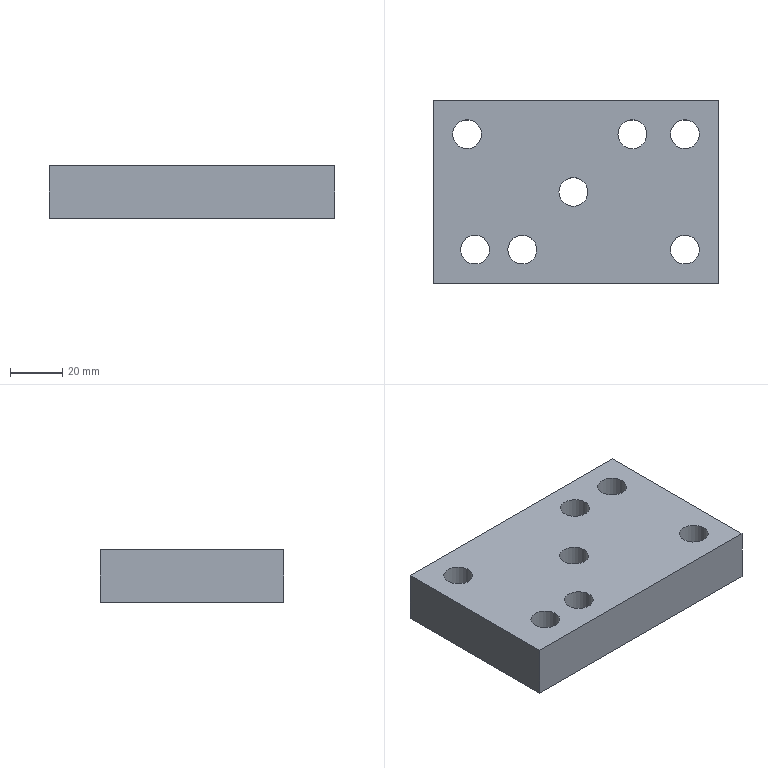Part | STEP file | 115_id2850_x_t | 1 solid | 13 faces | box 109 x 70 x 20 mm | volume 139295 mm3 | cylinder 7 | plane 6 | commonest cylinder face diameters 11 x7
STEP:
#1=CARTESIAN_POINT('',(0.,0.,0.));
#2=DIRECTION('',(0.,0.,1.));
#3=DIRECTION('',(1.,0.,0.));
#4=AXIS2_PLACEMENT_3D('',#1,#2,#3);
#5=CARTESIAN_POINT('',(1035.5,-161.,105.));
#6=VERTEX_POINT('',#5);
#7=CARTESIAN_POINT('',(1030.,-161.,105.));
#8=DIRECTION('',(0.,0.,1.));
#9=DIRECTION('',(1.,0.,0.));
#10=AXIS2_PLACEMENT_3D('',#7,#8,#9);
#11=CIRCLE('',#10,5.5);
#12=CARTESIAN_POINT('',(1030.,-162.5,105.));
#13=DIRECTION('',(0.,0.,1.));
#14=DIRECTION('',(-1.,0.,0.));
#15=AXIS2_PLACEMENT_3D('',#12,#13,#14);
#16=PLANE('',#15);
#17=CARTESIAN_POINT('',(0.,-1.5));
#18=DIRECTION('',(-1.,0.));
#19=AXIS2_PLACEMENT_2D('',#17,#18);
#20=CIRCLE('',#19,5.5);
#21=(GEOMETRIC_REPRESENTATION_CONTEXT(2)PARAMETRIC_REPRESENTATION_CONTEXT()REPRESENTATION_CONTEXT('',''));
#22=DEFINITIONAL_REPRESENTATION('',(#20),#21);
#23=PCURVE('',#16,#22);
#24=CARTESIAN_POINT('',(1030.,-161.,165.));
#25=DIRECTION('',(0.,0.,-1.));
#26=DIRECTION('',(1.,0.,0.));
#27=AXIS2_PLACEMENT_3D('',#24,#25,#26);
#28=CYLINDRICAL_SURFACE('',#27,5.5);
#29=CARTESIAN_POINT('',(6.283,60.));
#30=DIRECTION('',(-1.,0.));
#31=VECTOR('',#30,1.);
#32=LINE('',#29,#31);
#33=(GEOMETRIC_REPRESENTATION_CONTEXT(2)PARAMETRIC_REPRESENTATION_CONTEXT()REPRESENTATION_CONTEXT('',''));
#34=DEFINITIONAL_REPRESENTATION('',(#32),#33);
#35=PCURVE('',#28,#34);
#36=SURFACE_CURVE('',#11,(#23,#35),.PCURVE_S1.);
#37=EDGE_CURVE('',#6,#6,#36,.T.);
#38=ORIENTED_EDGE('',*,*,#37,.F.);
#39=EDGE_LOOP('',(#38));
#40=FACE_BOUND('',#39,.T.);
#41=CARTESIAN_POINT('',(1016.,-183.,105.));
#42=VERTEX_POINT('',#41);
#43=CARTESIAN_POINT('',(1005.,-183.,105.));
#44=VERTEX_POINT('',#43);
#45=CARTESIAN_POINT('',(1010.5,-183.,105.));
#46=DIRECTION('',(0.,0.,-1.));
#47=DIRECTION('',(1.,0.,0.));
#48=AXIS2_PLACEMENT_3D('',#45,#46,#47);
#49=CIRCLE('',#48,5.5);
#50=CARTESIAN_POINT('',(14.,20.5));
#51=CARTESIAN_POINT('',(14.,30.026));
#52=CARTESIAN_POINT('',(22.25,25.263));
#53=CARTESIAN_POINT('',(30.5,20.5));
#54=CARTESIAN_POINT('',(22.25,15.737));
#55=CARTESIAN_POINT('',(14.,10.974));
#56=CARTESIAN_POINT('',(14.,20.5));
#57=(BOUNDED_CURVE()B_SPLINE_CURVE(2,(#50,#51,#52,#53,#54,#55,#56),.UNSPECIFIED.,.T.,.F.)B_SPLINE_CURVE_WITH_KNOTS((1,2,2,2,2,1),(-2.094,0.,2.094,4.189,6.283,8.378),.UNSPECIFIED.)CURVE()GEOMETRIC_REPRESENTATION_ITEM()RATIONAL_B_SPLINE_CURVE((1.,0.5,1.,0.5,1.,0.5,1.))REPRESENTATION_ITEM(''));
#58=(GEOMETRIC_REPRESENTATION_CONTEXT(2)PARAMETRIC_REPRESENTATION_CONTEXT()REPRESENTATION_CONTEXT('',''));
#59=DEFINITIONAL_REPRESENTATION('',(#57),#58);
#60=PCURVE('',#16,#59);
#61=CARTESIAN_POINT('',(1010.5,-183.,90.));
#62=DIRECTION('',(0.,0.,1.));
#63=DIRECTION('',(-1.,0.,0.));
#64=AXIS2_PLACEMENT_3D('',#61,#62,#63);
#65=CYLINDRICAL_SURFACE('',#64,5.5);
#66=CARTESIAN_POINT('',(3.142,15.));
#67=DIRECTION('',(-1.,0.));
#68=VECTOR('',#67,1.);
#69=LINE('',#66,#68);
#70=(GEOMETRIC_REPRESENTATION_CONTEXT(2)PARAMETRIC_REPRESENTATION_CONTEXT()REPRESENTATION_CONTEXT('',''));
#71=DEFINITIONAL_REPRESENTATION('',(#69),#70);
#72=PCURVE('',#65,#71);
#73=SURFACE_CURVE('',#49,(#60,#72),.PCURVE_S1.);
#74=EDGE_CURVE('',#42,#44,#73,.T.);
#75=ORIENTED_EDGE('',*,*,#74,.T.);
#76=CARTESIAN_POINT('',(1010.5,-183.,105.));
#77=DIRECTION('',(0.,0.,-1.));
#78=DIRECTION('',(1.,0.,0.));
#79=AXIS2_PLACEMENT_3D('',#76,#77,#78);
#80=CIRCLE('',#79,5.5);
#81=CARTESIAN_POINT('',(14.,20.5));
#82=CARTESIAN_POINT('',(14.,30.026));
#83=CARTESIAN_POINT('',(22.25,25.263));
#84=CARTESIAN_POINT('',(30.5,20.5));
#85=CARTESIAN_POINT('',(22.25,15.737));
#86=CARTESIAN_POINT('',(14.,10.974));
#87=CARTESIAN_POINT('',(14.,20.5));
#88=(BOUNDED_CURVE()B_SPLINE_CURVE(2,(#81,#82,#83,#84,#85,#86,#87),.UNSPECIFIED.,.T.,.F.)B_SPLINE_CURVE_WITH_KNOTS((1,2,2,2,2,1),(-2.094,0.,2.094,4.189,6.283,8.378),.UNSPECIFIED.)CURVE()GEOMETRIC_REPRESENTATION_ITEM()RATIONAL_B_SPLINE_CURVE((1.,0.5,1.,0.5,1.,0.5,1.))REPRESENTATION_ITEM(''));
#89=(GEOMETRIC_REPRESENTATION_CONTEXT(2)PARAMETRIC_REPRESENTATION_CONTEXT()REPRESENTATION_CONTEXT('',''));
#90=DEFINITIONAL_REPRESENTATION('',(#88),#89);
#91=PCURVE('',#16,#90);
#92=CARTESIAN_POINT('',(9.425,15.));
#93=DIRECTION('',(-1.,0.));
#94=VECTOR('',#93,1.);
#95=LINE('',#92,#94);
#96=(GEOMETRIC_REPRESENTATION_CONTEXT(2)PARAMETRIC_REPRESENTATION_CONTEXT()REPRESENTATION_CONTEXT('',''));
#97=DEFINITIONAL_REPRESENTATION('',(#95),#96);
#98=PCURVE('',#65,#97);
#99=SURFACE_CURVE('',#80,(#91,#98),.PCURVE_S1.);
#100=EDGE_CURVE('',#44,#42,#99,.T.);
#101=ORIENTED_EDGE('',*,*,#100,.T.);
#102=EDGE_LOOP('',(#75,#101));
#103=FACE_BOUND('',#102,.T.);
#104=CARTESIAN_POINT('',(1078.,-139.,105.));
#105=VERTEX_POINT('',#104);
#106=CARTESIAN_POINT('',(1067.,-139.,105.));
#107=VERTEX_POINT('',#106);
#108=CARTESIAN_POINT('',(1072.5,-139.,105.));
#109=DIRECTION('',(0.,0.,-1.));
#110=DIRECTION('',(1.,0.,0.));
#111=AXIS2_PLACEMENT_3D('',#108,#109,#110);
#112=CIRCLE('',#111,5.5);
#113=CARTESIAN_POINT('',(-48.,-23.5));
#114=CARTESIAN_POINT('',(-48.,-13.974));
#115=CARTESIAN_POINT('',(-39.75,-18.737));
#116=CARTESIAN_POINT('',(-31.5,-23.5));
#117=CARTESIAN_POINT('',(-39.75,-28.263));
#118=CARTESIAN_POINT('',(-48.,-33.026));
#119=CARTESIAN_POINT('',(-48.,-23.5));
#120=(BOUNDED_CURVE()B_SPLINE_CURVE(2,(#113,#114,#115,#116,#117,#118,#119),.UNSPECIFIED.,.T.,.F.)B_SPLINE_CURVE_WITH_KNOTS((1,2,2,2,2,1),(-2.094,0.,2.094,4.189,6.283,8.378),.UNSPECIFIED.)CURVE()GEOMETRIC_REPRESENTATION_ITEM()RATIONAL_B_SPLINE_CURVE((1.,0.5,1.,0.5,1.,0.5,1.))REPRESENTATION_ITEM(''));
#121=(GEOMETRIC_REPRESENTATION_CONTEXT(2)PARAMETRIC_REPRESENTATION_CONTEXT()REPRESENTATION_CONTEXT('',''));
#122=DEFINITIONAL_REPRESENTATION('',(#120),#121);
#123=PCURVE('',#16,#122);
#124=CARTESIAN_POINT('',(1072.5,-139.,90.));
#125=DIRECTION('',(0.,0.,1.));
#126=DIRECTION('',(-1.,0.,0.));
#127=AXIS2_PLACEMENT_3D('',#124,#125,#126);
#128=CYLINDRICAL_SURFACE('',#127,5.5);
#129=CARTESIAN_POINT('',(3.142,15.));
#130=DIRECTION('',(-1.,0.));
#131=VECTOR('',#130,1.);
#132=LINE('',#129,#131);
#133=(GEOMETRIC_REPRESENTATION_CONTEXT(2)PARAMETRIC_REPRESENTATION_CONTEXT()REPRESENTATION_CONTEXT('',''));
#134=DEFINITIONAL_REPRESENTATION('',(#132),#133);
#135=PCURVE('',#128,#134);
#136=SURFACE_CURVE('',#112,(#123,#135),.PCURVE_S1.);
#137=EDGE_CURVE('',#105,#107,#136,.T.);
#138=ORIENTED_EDGE('',*,*,#137,.T.);
#139=CARTESIAN_POINT('',(1072.5,-139.,105.));
#140=DIRECTION('',(0.,0.,-1.));
#141=DIRECTION('',(1.,0.,0.));
#142=AXIS2_PLACEMENT_3D('',#139,#140,#141);
#143=CIRCLE('',#142,5.5);
#144=CARTESIAN_POINT('',(-48.,-23.5));
#145=CARTESIAN_POINT('',(-48.,-13.974));
#146=CARTESIAN_POINT('',(-39.75,-18.737));
#147=CARTESIAN_POINT('',(-31.5,-23.5));
#148=CARTESIAN_POINT('',(-39.75,-28.263));
#149=CARTESIAN_POINT('',(-48.,-33.026));
#150=CARTESIAN_POINT('',(-48.,-23.5));
#151=(BOUNDED_CURVE()B_SPLINE_CURVE(2,(#144,#145,#146,#147,#148,#149,#150),.UNSPECIFIED.,.T.,.F.)B_SPLINE_CURVE_WITH_KNOTS((1,2,2,2,2,1),(-2.094,0.,2.094,4.189,6.283,8.378),.UNSPECIFIED.)CURVE()GEOMETRIC_REPRESENTATION_ITEM()RATIONAL_B_SPLINE_CURVE((1.,0.5,1.,0.5,1.,0.5,1.))REPRESENTATION_ITEM(''));
#152=(GEOMETRIC_REPRESENTATION_CONTEXT(2)PARAMETRIC_REPRESENTATION_CONTEXT()REPRESENTATION_CONTEXT('',''));
#153=DEFINITIONAL_REPRESENTATION('',(#151),#152);
#154=PCURVE('',#16,#153);
#155=CARTESIAN_POINT('',(9.425,15.));
#156=DIRECTION('',(-1.,0.));
#157=VECTOR('',#156,1.);
#158=LINE('',#155,#157);
#159=(GEOMETRIC_REPRESENTATION_CONTEXT(2)PARAMETRIC_REPRESENTATION_CONTEXT()REPRESENTATION_CONTEXT('',''));
#160=DEFINITIONAL_REPRESENTATION('',(#158),#159);
#161=PCURVE('',#128,#160);
#162=SURFACE_CURVE('',#143,(#154,#161),.PCURVE_S1.);
#163=EDGE_CURVE('',#107,#105,#162,.T.);
#164=ORIENTED_EDGE('',*,*,#163,.T.);
#165=EDGE_LOOP('',(#138,#164));
#166=FACE_BOUND('',#165,.T.);
#167=CARTESIAN_POINT('',(998.,-183.,105.));
#168=VERTEX_POINT('',#167);
#169=CARTESIAN_POINT('',(987.,-183.,105.));
#170=VERTEX_POINT('',#169);
#171=CARTESIAN_POINT('',(992.5,-183.,105.));
#172=DIRECTION('',(0.,0.,-1.));
#173=DIRECTION('',(1.,0.,0.));
#174=AXIS2_PLACEMENT_3D('',#171,#172,#173);
#175=CIRCLE('',#174,5.5);
#176=CARTESIAN_POINT('',(32.,20.5));
#177=CARTESIAN_POINT('',(32.,30.026));
#178=CARTESIAN_POINT('',(40.25,25.263));
#179=CARTESIAN_POINT('',(48.5,20.5));
#180=CARTESIAN_POINT('',(40.25,15.737));
#181=CARTESIAN_POINT('',(32.,10.974));
#182=CARTESIAN_POINT('',(32.,20.5));
#183=(BOUNDED_CURVE()B_SPLINE_CURVE(2,(#176,#177,#178,#179,#180,#181,#182),.UNSPECIFIED.,.T.,.F.)B_SPLINE_CURVE_WITH_KNOTS((1,2,2,2,2,1),(-2.094,0.,2.094,4.189,6.283,8.378),.UNSPECIFIED.)CURVE()GEOMETRIC_REPRESENTATION_ITEM()RATIONAL_B_SPLINE_CURVE((1.,0.5,1.,0.5,1.,0.5,1.))REPRESENTATION_ITEM(''));
#184=(GEOMETRIC_REPRESENTATION_CONTEXT(2)PARAMETRIC_REPRESENTATION_CONTEXT()REPRESENTATION_CONTEXT('',''));
#185=DEFINITIONAL_REPRESENTATION('',(#183),#184);
#186=PCURVE('',#16,#185);
#187=CARTESIAN_POINT('',(992.5,-183.,90.));
#188=DIRECTION('',(0.,0.,1.));
#189=DIRECTION('',(-1.,0.,0.));
#190=AXIS2_PLACEMENT_3D('',#187,#188,#189);
#191=CYLINDRICAL_SURFACE('',#190,5.5);
#192=CARTESIAN_POINT('',(3.142,15.));
#193=DIRECTION('',(-1.,0.));
#194=VECTOR('',#193,1.);
#195=LINE('',#192,#194);
#196=(GEOMETRIC_REPRESENTATION_CONTEXT(2)PARAMETRIC_REPRESENTATION_CONTEXT()REPRESENTATION_CONTEXT('',''));
#197=DEFINITIONAL_REPRESENTATION('',(#195),#196);
#198=PCURVE('',#191,#197);
#199=SURFACE_CURVE('',#175,(#186,#198),.PCURVE_S1.);
#200=EDGE_CURVE('',#168,#170,#199,.T.);
#201=ORIENTED_EDGE('',*,*,#200,.T.);
#202=CARTESIAN_POINT('',(992.5,-183.,105.));
#203=DIRECTION('',(0.,0.,-1.));
#204=DIRECTION('',(1.,0.,0.));
#205=AXIS2_PLACEMENT_3D('',#202,#203,#204);
#206=CIRCLE('',#205,5.5);
#207=CARTESIAN_POINT('',(32.,20.5));
#208=CARTESIAN_POINT('',(32.,30.026));
#209=CARTESIAN_POINT('',(40.25,25.263));
#210=CARTESIAN_POINT('',(48.5,20.5));
#211=CARTESIAN_POINT('',(40.25,15.737));
#212=CARTESIAN_POINT('',(32.,10.974));
#213=CARTESIAN_POINT('',(32.,20.5));
#214=(BOUNDED_CURVE()B_SPLINE_CURVE(2,(#207,#208,#209,#210,#211,#212,#213),.UNSPECIFIED.,.T.,.F.)B_SPLINE_CURVE_WITH_KNOTS((1,2,2,2,2,1),(-2.094,0.,2.094,4.189,6.283,8.378),.UNSPECIFIED.)CURVE()GEOMETRIC_REPRESENTATION_ITEM()RATIONAL_B_SPLINE_CURVE((1.,0.5,1.,0.5,1.,0.5,1.))REPRESENTATION_ITEM(''));
#215=(GEOMETRIC_REPRESENTATION_CONTEXT(2)PARAMETRIC_REPRESENTATION_CONTEXT()REPRESENTATION_CONTEXT('',''));
#216=DEFINITIONAL_REPRESENTATION('',(#214),#215);
#217=PCURVE('',#16,#216);
#218=CARTESIAN_POINT('',(9.425,15.));
#219=DIRECTION('',(-1.,0.));
#220=VECTOR('',#219,1.);
#221=LINE('',#218,#220);
#222=(GEOMETRIC_REPRESENTATION_CONTEXT(2)PARAMETRIC_REPRESENTATION_CONTEXT()REPRESENTATION_CONTEXT('',''));
#223=DEFINITIONAL_REPRESENTATION('',(#221),#222);
#224=PCURVE('',#191,#223);
#225=SURFACE_CURVE('',#206,(#217,#224),.PCURVE_S1.);
#226=EDGE_CURVE('',#170,#168,#225,.T.);
#227=ORIENTED_EDGE('',*,*,#226,.T.);
#228=EDGE_LOOP('',(#201,#227));
#229=FACE_BOUND('',#228,.T.);
#230=CARTESIAN_POINT('',(1085.5,-196.,105.));
#231=VERTEX_POINT('',#230);
#232=CARTESIAN_POINT('',(976.5,-196.,105.));
#233=VERTEX_POINT('',#232);
#234=CARTESIAN_POINT('',(1030.,-196.,105.));
#235=DIRECTION('',(-1.,0.,0.));
#236=VECTOR('',#235,1.);
#237=LINE('',#234,#236);
#238=CARTESIAN_POINT('',(0.,33.5));
#239=DIRECTION('',(1.,0.));
#240=VECTOR('',#239,1.);
#241=LINE('',#238,#240);
#242=(GEOMETRIC_REPRESENTATION_CONTEXT(2)PARAMETRIC_REPRESENTATION_CONTEXT()REPRESENTATION_CONTEXT('',''));
#243=DEFINITIONAL_REPRESENTATION('',(#241),#242);
#244=PCURVE('',#16,#243);
#245=CARTESIAN_POINT('',(1030.,-196.,90.));
#246=DIRECTION('',(0.,-1.,0.));
#247=DIRECTION('',(0.,0.,1.));
#248=AXIS2_PLACEMENT_3D('',#245,#246,#247);
#249=PLANE('',#248);
#250=CARTESIAN_POINT('',(15.,0.));
#251=DIRECTION('',(0.,1.));
#252=VECTOR('',#251,1.);
#253=LINE('',#250,#252);
#254=(GEOMETRIC_REPRESENTATION_CONTEXT(2)PARAMETRIC_REPRESENTATION_CONTEXT()REPRESENTATION_CONTEXT('',''));
#255=DEFINITIONAL_REPRESENTATION('',(#253),#254);
#256=PCURVE('',#249,#255);
#257=SURFACE_CURVE('',#237,(#244,#256),.PCURVE_S1.);
#258=EDGE_CURVE('',#231,#233,#257,.T.);
#259=ORIENTED_EDGE('',*,*,#258,.F.);
#260=CARTESIAN_POINT('',(1085.5,-126.,105.));
#261=VERTEX_POINT('',#260);
#262=CARTESIAN_POINT('',(1085.5,-162.5,105.));
#263=DIRECTION('',(0.,-1.,0.));
#264=VECTOR('',#263,1.);
#265=LINE('',#262,#264);
#266=CARTESIAN_POINT('',(-55.5,0.));
#267=DIRECTION('',(0.,1.));
#268=VECTOR('',#267,1.);
#269=LINE('',#266,#268);
#270=(GEOMETRIC_REPRESENTATION_CONTEXT(2)PARAMETRIC_REPRESENTATION_CONTEXT()REPRESENTATION_CONTEXT('',''));
#271=DEFINITIONAL_REPRESENTATION('',(#269),#270);
#272=PCURVE('',#16,#271);
#273=CARTESIAN_POINT('',(1085.5,-162.5,90.));
#274=DIRECTION('',(1.,0.,0.));
#275=DIRECTION('',(0.,0.,1.));
#276=AXIS2_PLACEMENT_3D('',#273,#274,#275);
#277=PLANE('',#276);
#278=CARTESIAN_POINT('',(15.,0.));
#279=DIRECTION('',(0.,1.));
#280=VECTOR('',#279,1.);
#281=LINE('',#278,#280);
#282=(GEOMETRIC_REPRESENTATION_CONTEXT(2)PARAMETRIC_REPRESENTATION_CONTEXT()REPRESENTATION_CONTEXT('',''));
#283=DEFINITIONAL_REPRESENTATION('',(#281),#282);
#284=PCURVE('',#277,#283);
#285=SURFACE_CURVE('',#265,(#272,#284),.PCURVE_S1.);
#286=EDGE_CURVE('',#261,#231,#285,.T.);
#287=ORIENTED_EDGE('',*,*,#286,.F.);
#288=CARTESIAN_POINT('',(976.5,-126.,105.));
#289=VERTEX_POINT('',#288);
#290=CARTESIAN_POINT('',(1030.,-126.,105.));
#291=DIRECTION('',(1.,0.,0.));
#292=VECTOR('',#291,1.);
#293=LINE('',#290,#292);
#294=CARTESIAN_POINT('',(0.,-36.5));
#295=DIRECTION('',(-1.,0.));
#296=VECTOR('',#295,1.);
#297=LINE('',#294,#296);
#298=(GEOMETRIC_REPRESENTATION_CONTEXT(2)PARAMETRIC_REPRESENTATION_CONTEXT()REPRESENTATION_CONTEXT('',''));
#299=DEFINITIONAL_REPRESENTATION('',(#297),#298);
#300=PCURVE('',#16,#299);
#301=CARTESIAN_POINT('',(1030.,-126.,90.));
#302=DIRECTION('',(0.,1.,0.));
#303=DIRECTION('',(0.,0.,-1.));
#304=AXIS2_PLACEMENT_3D('',#301,#302,#303);
#305=PLANE('',#304);
#306=CARTESIAN_POINT('',(-15.,0.));
#307=DIRECTION('',(0.,-1.));
#308=VECTOR('',#307,1.);
#309=LINE('',#306,#308);
#310=(GEOMETRIC_REPRESENTATION_CONTEXT(2)PARAMETRIC_REPRESENTATION_CONTEXT()REPRESENTATION_CONTEXT('',''));
#311=DEFINITIONAL_REPRESENTATION('',(#309),#310);
#312=PCURVE('',#305,#311);
#313=SURFACE_CURVE('',#293,(#300,#312),.PCURVE_S1.);
#314=EDGE_CURVE('',#289,#261,#313,.T.);
#315=ORIENTED_EDGE('',*,*,#314,.F.);
#316=CARTESIAN_POINT('',(976.5,-162.5,105.));
#317=DIRECTION('',(0.,1.,0.));
#318=VECTOR('',#317,1.);
#319=LINE('',#316,#318);
#320=CARTESIAN_POINT('',(53.5,0.));
#321=DIRECTION('',(0.,-1.));
#322=VECTOR('',#321,1.);
#323=LINE('',#320,#322);
#324=(GEOMETRIC_REPRESENTATION_CONTEXT(2)PARAMETRIC_REPRESENTATION_CONTEXT()REPRESENTATION_CONTEXT('',''));
#325=DEFINITIONAL_REPRESENTATION('',(#323),#324);
#326=PCURVE('',#16,#325);
#327=CARTESIAN_POINT('',(976.5,-162.5,90.));
#328=DIRECTION('',(-1.,0.,0.));
#329=DIRECTION('',(0.,0.,-1.));
#330=AXIS2_PLACEMENT_3D('',#327,#328,#329);
#331=PLANE('',#330);
#332=CARTESIAN_POINT('',(-15.,0.));
#333=DIRECTION('',(0.,-1.));
#334=VECTOR('',#333,1.);
#335=LINE('',#332,#334);
#336=(GEOMETRIC_REPRESENTATION_CONTEXT(2)PARAMETRIC_REPRESENTATION_CONTEXT()REPRESENTATION_CONTEXT('',''));
#337=DEFINITIONAL_REPRESENTATION('',(#335),#336);
#338=PCURVE('',#331,#337);
#339=SURFACE_CURVE('',#319,(#326,#338),.PCURVE_S1.);
#340=EDGE_CURVE('',#233,#289,#339,.T.);
#341=ORIENTED_EDGE('',*,*,#340,.F.);
#342=EDGE_LOOP('',(#259,#287,#315,#341));
#343=FACE_BOUND('',#342,.T.);
#344=CARTESIAN_POINT('',(1078.,-183.,105.));
#345=VERTEX_POINT('',#344);
#346=CARTESIAN_POINT('',(1067.,-183.,105.));
#347=VERTEX_POINT('',#346);
#348=CARTESIAN_POINT('',(1072.5,-183.,105.));
#349=DIRECTION('',(0.,0.,-1.));
#350=DIRECTION('',(1.,0.,0.));
#351=AXIS2_PLACEMENT_3D('',#348,#349,#350);
#352=CIRCLE('',#351,5.5);
#353=CARTESIAN_POINT('',(-48.,20.5));
#354=CARTESIAN_POINT('',(-48.,30.026));
#355=CARTESIAN_POINT('',(-39.75,25.263));
#356=CARTESIAN_POINT('',(-31.5,20.5));
#357=CARTESIAN_POINT('',(-39.75,15.737));
#358=CARTESIAN_POINT('',(-48.,10.974));
#359=CARTESIAN_POINT('',(-48.,20.5));
#360=(BOUNDED_CURVE()B_SPLINE_CURVE(2,(#353,#354,#355,#356,#357,#358,#359),.UNSPECIFIED.,.T.,.F.)B_SPLINE_CURVE_WITH_KNOTS((1,2,2,2,2,1),(-2.094,0.,2.094,4.189,6.283,8.378),.UNSPECIFIED.)CURVE()GEOMETRIC_REPRESENTATION_ITEM()RATIONAL_B_SPLINE_CURVE((1.,0.5,1.,0.5,1.,0.5,1.))REPRESENTATION_ITEM(''));
#361=(GEOMETRIC_REPRESENTATION_CONTEXT(2)PARAMETRIC_REPRESENTATION_CONTEXT()REPRESENTATION_CONTEXT('',''));
#362=DEFINITIONAL_REPRESENTATION('',(#360),#361);
#363=PCURVE('',#16,#362);
#364=CARTESIAN_POINT('',(1072.5,-183.,90.));
#365=DIRECTION('',(0.,0.,1.));
#366=DIRECTION('',(-1.,0.,0.));
#367=AXIS2_PLACEMENT_3D('',#364,#365,#366);
#368=CYLINDRICAL_SURFACE('',#367,5.5);
#369=CARTESIAN_POINT('',(3.142,15.));
#370=DIRECTION('',(-1.,0.));
#371=VECTOR('',#370,1.);
#372=LINE('',#369,#371);
#373=(GEOMETRIC_REPRESENTATION_CONTEXT(2)PARAMETRIC_REPRESENTATION_CONTEXT()REPRESENTATION_CONTEXT('',''));
#374=DEFINITIONAL_REPRESENTATION('',(#372),#373);
#375=PCURVE('',#368,#374);
#376=SURFACE_CURVE('',#352,(#363,#375),.PCURVE_S1.);
#377=EDGE_CURVE('',#345,#347,#376,.T.);
#378=ORIENTED_EDGE('',*,*,#377,.T.);
#379=CARTESIAN_POINT('',(1072.5,-183.,105.));
#380=DIRECTION('',(0.,0.,-1.));
#381=DIRECTION('',(1.,0.,0.));
#382=AXIS2_PLACEMENT_3D('',#379,#380,#381);
#383=CIRCLE('',#382,5.5);
#384=CARTESIAN_POINT('',(-48.,20.5));
#385=CARTESIAN_POINT('',(-48.,30.026));
#386=CARTESIAN_POINT('',(-39.75,25.263));
#387=CARTESIAN_POINT('',(-31.5,20.5));
#388=CARTESIAN_POINT('',(-39.75,15.737));
#389=CARTESIAN_POINT('',(-48.,10.974));
#390=CARTESIAN_POINT('',(-48.,20.5));
#391=(BOUNDED_CURVE()B_SPLINE_CURVE(2,(#384,#385,#386,#387,#388,#389,#390),.UNSPECIFIED.,.T.,.F.)B_SPLINE_CURVE_WITH_KNOTS((1,2,2,2,2,1),(-2.094,0.,2.094,4.189,6.283,8.378),.UNSPECIFIED.)CURVE()GEOMETRIC_REPRESENTATION_ITEM()RATIONAL_B_SPLINE_CURVE((1.,0.5,1.,0.5,1.,0.5,1.))REPRESENTATION_ITEM(''));
#392=(GEOMETRIC_REPRESENTATION_CONTEXT(2)PARAMETRIC_REPRESENTATION_CONTEXT()REPRESENTATION_CONTEXT('',''));
#393=DEFINITIONAL_REPRESENTATION('',(#391),#392);
#394=PCURVE('',#16,#393);
#395=CARTESIAN_POINT('',(9.425,15.));
#396=DIRECTION('',(-1.,0.));
#397=VECTOR('',#396,1.);
#398=LINE('',#395,#397);
#399=(GEOMETRIC_REPRESENTATION_CONTEXT(2)PARAMETRIC_REPRESENTATION_CONTEXT()REPRESENTATION_CONTEXT('',''));
#400=DEFINITIONAL_REPRESENTATION('',(#398),#399);
#401=PCURVE('',#368,#400);
#402=SURFACE_CURVE('',#383,(#394,#401),.PCURVE_S1.);
#403=EDGE_CURVE('',#347,#345,#402,.T.);
#404=ORIENTED_EDGE('',*,*,#403,.T.);
#405=EDGE_LOOP('',(#378,#404));
#406=FACE_BOUND('',#405,.T.);
#407=CARTESIAN_POINT('',(995.,-139.,105.));
#408=VERTEX_POINT('',#407);
#409=CARTESIAN_POINT('',(984.,-139.,105.));
#410=VERTEX_POINT('',#409);
#411=CARTESIAN_POINT('',(989.5,-139.,105.));
#412=DIRECTION('',(0.,0.,-1.));
#413=DIRECTION('',(1.,0.,0.));
#414=AXIS2_PLACEMENT_3D('',#411,#412,#413);
#415=CIRCLE('',#414,5.5);
#416=CARTESIAN_POINT('',(35.,-23.5));
#417=CARTESIAN_POINT('',(35.,-13.974));
#418=CARTESIAN_POINT('',(43.25,-18.737));
#419=CARTESIAN_POINT('',(51.5,-23.5));
#420=CARTESIAN_POINT('',(43.25,-28.263));
#421=CARTESIAN_POINT('',(35.,-33.026));
#422=CARTESIAN_POINT('',(35.,-23.5));
#423=(BOUNDED_CURVE()B_SPLINE_CURVE(2,(#416,#417,#418,#419,#420,#421,#422),.UNSPECIFIED.,.T.,.F.)B_SPLINE_CURVE_WITH_KNOTS((1,2,2,2,2,1),(-2.094,0.,2.094,4.189,6.283,8.378),.UNSPECIFIED.)CURVE()GEOMETRIC_REPRESENTATION_ITEM()RATIONAL_B_SPLINE_CURVE((1.,0.5,1.,0.5,1.,0.5,1.))REPRESENTATION_ITEM(''));
#424=(GEOMETRIC_REPRESENTATION_CONTEXT(2)PARAMETRIC_REPRESENTATION_CONTEXT()REPRESENTATION_CONTEXT('',''));
#425=DEFINITIONAL_REPRESENTATION('',(#423),#424);
#426=PCURVE('',#16,#425);
#427=CARTESIAN_POINT('',(989.5,-139.,90.));
#428=DIRECTION('',(0.,0.,1.));
#429=DIRECTION('',(-1.,0.,0.));
#430=AXIS2_PLACEMENT_3D('',#427,#428,#429);
#431=CYLINDRICAL_SURFACE('',#430,5.5);
#432=CARTESIAN_POINT('',(3.142,15.));
#433=DIRECTION('',(-1.,0.));
#434=VECTOR('',#433,1.);
#435=LINE('',#432,#434);
#436=(GEOMETRIC_REPRESENTATION_CONTEXT(2)PARAMETRIC_REPRESENTATION_CONTEXT()REPRESENTATION_CONTEXT('',''));
#437=DEFINITIONAL_REPRESENTATION('',(#435),#436);
#438=PCURVE('',#431,#437);
#439=SURFACE_CURVE('',#415,(#426,#438),.PCURVE_S1.);
#440=EDGE_CURVE('',#408,#410,#439,.T.);
#441=ORIENTED_EDGE('',*,*,#440,.T.);
#442=CARTESIAN_POINT('',(989.5,-139.,105.));
#443=DIRECTION('',(0.,0.,-1.));
#444=DIRECTION('',(1.,0.,0.));
#445=AXIS2_PLACEMENT_3D('',#442,#443,#444);
#446=CIRCLE('',#445,5.5);
#447=CARTESIAN_POINT('',(35.,-23.5));
#448=CARTESIAN_POINT('',(35.,-13.974));
#449=CARTESIAN_POINT('',(43.25,-18.737));
#450=CARTESIAN_POINT('',(51.5,-23.5));
#451=CARTESIAN_POINT('',(43.25,-28.263));
#452=CARTESIAN_POINT('',(35.,-33.026));
#453=CARTESIAN_POINT('',(35.,-23.5));
#454=(BOUNDED_CURVE()B_SPLINE_CURVE(2,(#447,#448,#449,#450,#451,#452,#453),.UNSPECIFIED.,.T.,.F.)B_SPLINE_CURVE_WITH_KNOTS((1,2,2,2,2,1),(-2.094,0.,2.094,4.189,6.283,8.378),.UNSPECIFIED.)CURVE()GEOMETRIC_REPRESENTATION_ITEM()RATIONAL_B_SPLINE_CURVE((1.,0.5,1.,0.5,1.,0.5,1.))REPRESENTATION_ITEM(''));
#455=(GEOMETRIC_REPRESENTATION_CONTEXT(2)PARAMETRIC_REPRESENTATION_CONTEXT()REPRESENTATION_CONTEXT('',''));
#456=DEFINITIONAL_REPRESENTATION('',(#454),#455);
#457=PCURVE('',#16,#456);
#458=CARTESIAN_POINT('',(9.425,15.));
#459=DIRECTION('',(-1.,0.));
#460=VECTOR('',#459,1.);
#461=LINE('',#458,#460);
#462=(GEOMETRIC_REPRESENTATION_CONTEXT(2)PARAMETRIC_REPRESENTATION_CONTEXT()REPRESENTATION_CONTEXT('',''));
#463=DEFINITIONAL_REPRESENTATION('',(#461),#462);
#464=PCURVE('',#431,#463);
#465=SURFACE_CURVE('',#446,(#457,#464),.PCURVE_S1.);
#466=EDGE_CURVE('',#410,#408,#465,.T.);
#467=ORIENTED_EDGE('',*,*,#466,.T.);
#468=EDGE_LOOP('',(#441,#467));
#469=FACE_BOUND('',#468,.T.);
#470=CARTESIAN_POINT('',(1058.,-139.,105.));
#471=VERTEX_POINT('',#470);
#472=CARTESIAN_POINT('',(1047.,-139.,105.));
#473=VERTEX_POINT('',#472);
#474=CARTESIAN_POINT('',(1052.5,-139.,105.));
#475=DIRECTION('',(0.,0.,-1.));
#476=DIRECTION('',(1.,0.,0.));
#477=AXIS2_PLACEMENT_3D('',#474,#475,#476);
#478=CIRCLE('',#477,5.5);
#479=CARTESIAN_POINT('',(-28.,-23.5));
#480=CARTESIAN_POINT('',(-28.,-13.974));
#481=CARTESIAN_POINT('',(-19.75,-18.737));
#482=CARTESIAN_POINT('',(-11.5,-23.5));
#483=CARTESIAN_POINT('',(-19.75,-28.263));
#484=CARTESIAN_POINT('',(-28.,-33.026));
#485=CARTESIAN_POINT('',(-28.,-23.5));
#486=(BOUNDED_CURVE()B_SPLINE_CURVE(2,(#479,#480,#481,#482,#483,#484,#485),.UNSPECIFIED.,.T.,.F.)B_SPLINE_CURVE_WITH_KNOTS((1,2,2,2,2,1),(-2.094,0.,2.094,4.189,6.283,8.378),.UNSPECIFIED.)CURVE()GEOMETRIC_REPRESENTATION_ITEM()RATIONAL_B_SPLINE_CURVE((1.,0.5,1.,0.5,1.,0.5,1.))REPRESENTATION_ITEM(''));
#487=(GEOMETRIC_REPRESENTATION_CONTEXT(2)PARAMETRIC_REPRESENTATION_CONTEXT()REPRESENTATION_CONTEXT('',''));
#488=DEFINITIONAL_REPRESENTATION('',(#486),#487);
#489=PCURVE('',#16,#488);
#490=CARTESIAN_POINT('',(1052.5,-139.,90.));
#491=DIRECTION('',(0.,0.,1.));
#492=DIRECTION('',(-1.,0.,0.));
#493=AXIS2_PLACEMENT_3D('',#490,#491,#492);
#494=CYLINDRICAL_SURFACE('',#493,5.5);
#495=CARTESIAN_POINT('',(3.142,15.));
#496=DIRECTION('',(-1.,0.));
#497=VECTOR('',#496,1.);
#498=LINE('',#495,#497);
#499=(GEOMETRIC_REPRESENTATION_CONTEXT(2)PARAMETRIC_REPRESENTATION_CONTEXT()REPRESENTATION_CONTEXT('',''));
#500=DEFINITIONAL_REPRESENTATION('',(#498),#499);
#501=PCURVE('',#494,#500);
#502=SURFACE_CURVE('',#478,(#489,#501),.PCURVE_S1.);
#503=EDGE_CURVE('',#471,#473,#502,.T.);
#504=ORIENTED_EDGE('',*,*,#503,.T.);
#505=CARTESIAN_POINT('',(1052.5,-139.,105.));
#506=DIRECTION('',(0.,0.,-1.));
#507=DIRECTION('',(1.,0.,0.));
#508=AXIS2_PLACEMENT_3D('',#505,#506,#507);
#509=CIRCLE('',#508,5.5);
#510=CARTESIAN_POINT('',(-28.,-23.5));
#511=CARTESIAN_POINT('',(-28.,-13.974));
#512=CARTESIAN_POINT('',(-19.75,-18.737));
#513=CARTESIAN_POINT('',(-11.5,-23.5));
#514=CARTESIAN_POINT('',(-19.75,-28.263));
#515=CARTESIAN_POINT('',(-28.,-33.026));
#516=CARTESIAN_POINT('',(-28.,-23.5));
#517=(BOUNDED_CURVE()B_SPLINE_CURVE(2,(#510,#511,#512,#513,#514,#515,#516),.UNSPECIFIED.,.T.,.F.)B_SPLINE_CURVE_WITH_KNOTS((1,2,2,2,2,1),(-2.094,0.,2.094,4.189,6.283,8.378),.UNSPECIFIED.)CURVE()GEOMETRIC_REPRESENTATION_ITEM()RATIONAL_B_SPLINE_CURVE((1.,0.5,1.,0.5,1.,0.5,1.))REPRESENTATION_ITEM(''));
#518=(GEOMETRIC_REPRESENTATION_CONTEXT(2)PARAMETRIC_REPRESENTATION_CONTEXT()REPRESENTATION_CONTEXT('',''));
#519=DEFINITIONAL_REPRESENTATION('',(#517),#518);
#520=PCURVE('',#16,#519);
#521=CARTESIAN_POINT('',(9.425,15.));
#522=DIRECTION('',(-1.,0.));
#523=VECTOR('',#522,1.);
#524=LINE('',#521,#523);
#525=(GEOMETRIC_REPRESENTATION_CONTEXT(2)PARAMETRIC_REPRESENTATION_CONTEXT()REPRESENTATION_CONTEXT('',''));
#526=DEFINITIONAL_REPRESENTATION('',(#524),#525);
#527=PCURVE('',#494,#526);
#528=SURFACE_CURVE('',#509,(#520,#527),.PCURVE_S1.);
#529=EDGE_CURVE('',#473,#471,#528,.T.);
#530=ORIENTED_EDGE('',*,*,#529,.T.);
#531=EDGE_LOOP('',(#504,#530));
#532=FACE_BOUND('',#531,.T.);
#533=ADVANCED_FACE('',(#40,#103,#166,#229,#343,#406,#469,#532),#16,.T.);
#534=CARTESIAN_POINT('',(1024.5,-161.,85.));
#535=VERTEX_POINT('',#534);
#536=CARTESIAN_POINT('',(1035.5,-161.,85.));
#537=VERTEX_POINT('',#536);
#538=CARTESIAN_POINT('',(1030.,-161.,85.));
#539=DIRECTION('',(0.,0.,-1.));
#540=DIRECTION('',(-1.,0.,0.));
#541=AXIS2_PLACEMENT_3D('',#538,#539,#540);
#542=CIRCLE('',#541,5.5);
#543=CARTESIAN_POINT('',(1030.,-162.5,85.));
#544=DIRECTION('',(0.,0.,-1.));
#545=DIRECTION('',(1.,0.,0.));
#546=AXIS2_PLACEMENT_3D('',#543,#544,#545);
#547=PLANE('',#546);
#548=CARTESIAN_POINT('',(0.,-1.5));
#549=DIRECTION('',(-1.,0.));
#550=AXIS2_PLACEMENT_2D('',#548,#549);
#551=CIRCLE('',#550,5.5);
#552=(GEOMETRIC_REPRESENTATION_CONTEXT(2)PARAMETRIC_REPRESENTATION_CONTEXT()REPRESENTATION_CONTEXT('',''));
#553=DEFINITIONAL_REPRESENTATION('',(#551),#552);
#554=PCURVE('',#547,#553);
#555=CARTESIAN_POINT('',(3.142,80.));
#556=DIRECTION('',(1.,0.));
#557=VECTOR('',#556,1.);
#558=LINE('',#555,#557);
#559=(GEOMETRIC_REPRESENTATION_CONTEXT(2)PARAMETRIC_REPRESENTATION_CONTEXT()REPRESENTATION_CONTEXT('',''));
#560=DEFINITIONAL_REPRESENTATION('',(#558),#559);
#561=PCURVE('',#28,#560);
#562=SURFACE_CURVE('',#542,(#554,#561),.PCURVE_S1.);
#563=EDGE_CURVE('',#535,#537,#562,.T.);
#564=ORIENTED_EDGE('',*,*,#563,.F.);
#565=CARTESIAN_POINT('',(1030.,-161.,85.));
#566=DIRECTION('',(0.,0.,-1.));
#567=DIRECTION('',(-1.,0.,0.));
#568=AXIS2_PLACEMENT_3D('',#565,#566,#567);
#569=CIRCLE('',#568,5.5);
#570=CARTESIAN_POINT('',(0.,-1.5));
#571=DIRECTION('',(-1.,0.));
#572=AXIS2_PLACEMENT_2D('',#570,#571);
#573=CIRCLE('',#572,5.5);
#574=(GEOMETRIC_REPRESENTATION_CONTEXT(2)PARAMETRIC_REPRESENTATION_CONTEXT()REPRESENTATION_CONTEXT('',''));
#575=DEFINITIONAL_REPRESENTATION('',(#573),#574);
#576=PCURVE('',#547,#575);
#577=CARTESIAN_POINT('',(-3.142,80.));
#578=DIRECTION('',(1.,0.));
#579=VECTOR('',#578,1.);
#580=LINE('',#577,#579);
#581=(GEOMETRIC_REPRESENTATION_CONTEXT(2)PARAMETRIC_REPRESENTATION_CONTEXT()REPRESENTATION_CONTEXT('',''));
#582=DEFINITIONAL_REPRESENTATION('',(#580),#581);
#583=PCURVE('',#28,#582);
#584=SURFACE_CURVE('',#569,(#576,#583),.PCURVE_S1.);
#585=EDGE_CURVE('',#537,#535,#584,.T.);
#586=ORIENTED_EDGE('',*,*,#585,.F.);
#587=EDGE_LOOP('',(#564,#586));
#588=FACE_BOUND('',#587,.T.);
#589=CARTESIAN_POINT('',(1005.,-183.,85.));
#590=VERTEX_POINT('',#589);
#591=CARTESIAN_POINT('',(1010.5,-183.,85.));
#592=DIRECTION('',(0.,0.,1.));
#593=DIRECTION('',(-1.,0.,0.));
#594=AXIS2_PLACEMENT_3D('',#591,#592,#593);
#595=CIRCLE('',#594,5.5);
#596=CARTESIAN_POINT('',(-25.,20.5));
#597=CARTESIAN_POINT('',(-25.,30.026));
#598=CARTESIAN_POINT('',(-16.75,25.263));
#599=CARTESIAN_POINT('',(-8.5,20.5));
#600=CARTESIAN_POINT('',(-16.75,15.737));
#601=CARTESIAN_POINT('',(-25.,10.974));
#602=CARTESIAN_POINT('',(-25.,20.5));
#603=(BOUNDED_CURVE()B_SPLINE_CURVE(2,(#596,#597,#598,#599,#600,#601,#602),.UNSPECIFIED.,.T.,.F.)B_SPLINE_CURVE_WITH_KNOTS((1,2,2,2,2,1),(-2.094,0.,2.094,4.189,6.283,8.378),.UNSPECIFIED.)CURVE()GEOMETRIC_REPRESENTATION_ITEM()RATIONAL_B_SPLINE_CURVE((1.,0.5,1.,0.5,1.,0.5,1.))REPRESENTATION_ITEM(''));
#604=(GEOMETRIC_REPRESENTATION_CONTEXT(2)PARAMETRIC_REPRESENTATION_CONTEXT()REPRESENTATION_CONTEXT('',''));
#605=DEFINITIONAL_REPRESENTATION('',(#603),#604);
#606=PCURVE('',#547,#605);
#607=CARTESIAN_POINT('',(0.,-5.));
#608=DIRECTION('',(1.,0.));
#609=VECTOR('',#608,1.);
#610=LINE('',#607,#609);
#611=(GEOMETRIC_REPRESENTATION_CONTEXT(2)PARAMETRIC_REPRESENTATION_CONTEXT()REPRESENTATION_CONTEXT('',''));
#612=DEFINITIONAL_REPRESENTATION('',(#610),#611);
#613=PCURVE('',#65,#612);
#614=SURFACE_CURVE('',#595,(#606,#613),.PCURVE_S1.);
#615=EDGE_CURVE('',#590,#590,#614,.T.);
#616=ORIENTED_EDGE('',*,*,#615,.T.);
#617=EDGE_LOOP('',(#616));
#618=FACE_BOUND('',#617,.T.);
#619=CARTESIAN_POINT('',(1067.,-139.,85.));
#620=VERTEX_POINT('',#619);
#621=CARTESIAN_POINT('',(1072.5,-139.,85.));
#622=DIRECTION('',(0.,0.,1.));
#623=DIRECTION('',(-1.,0.,0.));
#624=AXIS2_PLACEMENT_3D('',#621,#622,#623);
#625=CIRCLE('',#624,5.5);
#626=CARTESIAN_POINT('',(37.,-23.5));
#627=CARTESIAN_POINT('',(37.,-13.974));
#628=CARTESIAN_POINT('',(45.25,-18.737));
#629=CARTESIAN_POINT('',(53.5,-23.5));
#630=CARTESIAN_POINT('',(45.25,-28.263));
#631=CARTESIAN_POINT('',(37.,-33.026));
#632=CARTESIAN_POINT('',(37.,-23.5));
#633=(BOUNDED_CURVE()B_SPLINE_CURVE(2,(#626,#627,#628,#629,#630,#631,#632),.UNSPECIFIED.,.T.,.F.)B_SPLINE_CURVE_WITH_KNOTS((1,2,2,2,2,1),(-2.094,0.,2.094,4.189,6.283,8.378),.UNSPECIFIED.)CURVE()GEOMETRIC_REPRESENTATION_ITEM()RATIONAL_B_SPLINE_CURVE((1.,0.5,1.,0.5,1.,0.5,1.))REPRESENTATION_ITEM(''));
#634=(GEOMETRIC_REPRESENTATION_CONTEXT(2)PARAMETRIC_REPRESENTATION_CONTEXT()REPRESENTATION_CONTEXT('',''));
#635=DEFINITIONAL_REPRESENTATION('',(#633),#634);
#636=PCURVE('',#547,#635);
#637=CARTESIAN_POINT('',(0.,-5.));
#638=DIRECTION('',(1.,0.));
#639=VECTOR('',#638,1.);
#640=LINE('',#637,#639);
#641=(GEOMETRIC_REPRESENTATION_CONTEXT(2)PARAMETRIC_REPRESENTATION_CONTEXT()REPRESENTATION_CONTEXT('',''));
#642=DEFINITIONAL_REPRESENTATION('',(#640),#641);
#643=PCURVE('',#128,#642);
#644=SURFACE_CURVE('',#625,(#636,#643),.PCURVE_S1.);
#645=EDGE_CURVE('',#620,#620,#644,.T.);
#646=ORIENTED_EDGE('',*,*,#645,.T.);
#647=EDGE_LOOP('',(#646));
#648=FACE_BOUND('',#647,.T.);
#649=CARTESIAN_POINT('',(987.,-183.,85.));
#650=VERTEX_POINT('',#649);
#651=CARTESIAN_POINT('',(992.5,-183.,85.));
#652=DIRECTION('',(0.,0.,1.));
#653=DIRECTION('',(-1.,0.,0.));
#654=AXIS2_PLACEMENT_3D('',#651,#652,#653);
#655=CIRCLE('',#654,5.5);
#656=CARTESIAN_POINT('',(-43.,20.5));
#657=CARTESIAN_POINT('',(-43.,30.026));
#658=CARTESIAN_POINT('',(-34.75,25.263));
#659=CARTESIAN_POINT('',(-26.5,20.5));
#660=CARTESIAN_POINT('',(-34.75,15.737));
#661=CARTESIAN_POINT('',(-43.,10.974));
#662=CARTESIAN_POINT('',(-43.,20.5));
#663=(BOUNDED_CURVE()B_SPLINE_CURVE(2,(#656,#657,#658,#659,#660,#661,#662),.UNSPECIFIED.,.T.,.F.)B_SPLINE_CURVE_WITH_KNOTS((1,2,2,2,2,1),(-2.094,0.,2.094,4.189,6.283,8.378),.UNSPECIFIED.)CURVE()GEOMETRIC_REPRESENTATION_ITEM()RATIONAL_B_SPLINE_CURVE((1.,0.5,1.,0.5,1.,0.5,1.))REPRESENTATION_ITEM(''));
#664=(GEOMETRIC_REPRESENTATION_CONTEXT(2)PARAMETRIC_REPRESENTATION_CONTEXT()REPRESENTATION_CONTEXT('',''));
#665=DEFINITIONAL_REPRESENTATION('',(#663),#664);
#666=PCURVE('',#547,#665);
#667=CARTESIAN_POINT('',(0.,-5.));
#668=DIRECTION('',(1.,0.));
#669=VECTOR('',#668,1.);
#670=LINE('',#667,#669);
#671=(GEOMETRIC_REPRESENTATION_CONTEXT(2)PARAMETRIC_REPRESENTATION_CONTEXT()REPRESENTATION_CONTEXT('',''));
#672=DEFINITIONAL_REPRESENTATION('',(#670),#671);
#673=PCURVE('',#191,#672);
#674=SURFACE_CURVE('',#655,(#666,#673),.PCURVE_S1.);
#675=EDGE_CURVE('',#650,#650,#674,.T.);
#676=ORIENTED_EDGE('',*,*,#675,.T.);
#677=EDGE_LOOP('',(#676));
#678=FACE_BOUND('',#677,.T.);
#679=CARTESIAN_POINT('',(1085.5,-196.,85.));
#680=VERTEX_POINT('',#679);
#681=CARTESIAN_POINT('',(1085.5,-126.,85.));
#682=VERTEX_POINT('',#681);
#683=CARTESIAN_POINT('',(1085.5,-162.5,85.));
#684=DIRECTION('',(0.,1.,0.));
#685=VECTOR('',#684,1.);
#686=LINE('',#683,#685);
#687=CARTESIAN_POINT('',(55.5,0.));
#688=DIRECTION('',(0.,-1.));
#689=VECTOR('',#688,1.);
#690=LINE('',#687,#689);
#691=(GEOMETRIC_REPRESENTATION_CONTEXT(2)PARAMETRIC_REPRESENTATION_CONTEXT()REPRESENTATION_CONTEXT('',''));
#692=DEFINITIONAL_REPRESENTATION('',(#690),#691);
#693=PCURVE('',#547,#692);
#694=CARTESIAN_POINT('',(-5.,0.));
#695=DIRECTION('',(0.,-1.));
#696=VECTOR('',#695,1.);
#697=LINE('',#694,#696);
#698=(GEOMETRIC_REPRESENTATION_CONTEXT(2)PARAMETRIC_REPRESENTATION_CONTEXT()REPRESENTATION_CONTEXT('',''));
#699=DEFINITIONAL_REPRESENTATION('',(#697),#698);
#700=PCURVE('',#277,#699);
#701=SURFACE_CURVE('',#686,(#693,#700),.PCURVE_S1.);
#702=EDGE_CURVE('',#680,#682,#701,.T.);
#703=ORIENTED_EDGE('',*,*,#702,.F.);
#704=CARTESIAN_POINT('',(976.5,-196.,85.));
#705=VERTEX_POINT('',#704);
#706=CARTESIAN_POINT('',(1030.,-196.,85.));
#707=DIRECTION('',(1.,0.,0.));
#708=VECTOR('',#707,1.);
#709=LINE('',#706,#708);
#710=CARTESIAN_POINT('',(0.,33.5));
#711=DIRECTION('',(1.,0.));
#712=VECTOR('',#711,1.);
#713=LINE('',#710,#712);
#714=(GEOMETRIC_REPRESENTATION_CONTEXT(2)PARAMETRIC_REPRESENTATION_CONTEXT()REPRESENTATION_CONTEXT('',''));
#715=DEFINITIONAL_REPRESENTATION('',(#713),#714);
#716=PCURVE('',#547,#715);
#717=CARTESIAN_POINT('',(-5.,0.));
#718=DIRECTION('',(0.,-1.));
#719=VECTOR('',#718,1.);
#720=LINE('',#717,#719);
#721=(GEOMETRIC_REPRESENTATION_CONTEXT(2)PARAMETRIC_REPRESENTATION_CONTEXT()REPRESENTATION_CONTEXT('',''));
#722=DEFINITIONAL_REPRESENTATION('',(#720),#721);
#723=PCURVE('',#249,#722);
#724=SURFACE_CURVE('',#709,(#716,#723),.PCURVE_S1.);
#725=EDGE_CURVE('',#705,#680,#724,.T.);
#726=ORIENTED_EDGE('',*,*,#725,.F.);
#727=CARTESIAN_POINT('',(976.5,-126.,85.));
#728=VERTEX_POINT('',#727);
#729=CARTESIAN_POINT('',(976.5,-162.5,85.));
#730=DIRECTION('',(0.,-1.,0.));
#731=VECTOR('',#730,1.);
#732=LINE('',#729,#731);
#733=CARTESIAN_POINT('',(-53.5,0.));
#734=DIRECTION('',(0.,1.));
#735=VECTOR('',#734,1.);
#736=LINE('',#733,#735);
#737=(GEOMETRIC_REPRESENTATION_CONTEXT(2)PARAMETRIC_REPRESENTATION_CONTEXT()REPRESENTATION_CONTEXT('',''));
#738=DEFINITIONAL_REPRESENTATION('',(#736),#737);
#739=PCURVE('',#547,#738);
#740=CARTESIAN_POINT('',(5.,0.));
#741=DIRECTION('',(0.,1.));
#742=VECTOR('',#741,1.);
#743=LINE('',#740,#742);
#744=(GEOMETRIC_REPRESENTATION_CONTEXT(2)PARAMETRIC_REPRESENTATION_CONTEXT()REPRESENTATION_CONTEXT('',''));
#745=DEFINITIONAL_REPRESENTATION('',(#743),#744);
#746=PCURVE('',#331,#745);
#747=SURFACE_CURVE('',#732,(#739,#746),.PCURVE_S1.);
#748=EDGE_CURVE('',#728,#705,#747,.T.);
#749=ORIENTED_EDGE('',*,*,#748,.F.);
#750=CARTESIAN_POINT('',(1030.,-126.,85.));
#751=DIRECTION('',(-1.,0.,0.));
#752=VECTOR('',#751,1.);
#753=LINE('',#750,#752);
#754=CARTESIAN_POINT('',(0.,-36.5));
#755=DIRECTION('',(-1.,0.));
#756=VECTOR('',#755,1.);
#757=LINE('',#754,#756);
#758=(GEOMETRIC_REPRESENTATION_CONTEXT(2)PARAMETRIC_REPRESENTATION_CONTEXT()REPRESENTATION_CONTEXT('',''));
#759=DEFINITIONAL_REPRESENTATION('',(#757),#758);
#760=PCURVE('',#547,#759);
#761=CARTESIAN_POINT('',(5.,0.));
#762=DIRECTION('',(0.,1.));
#763=VECTOR('',#762,1.);
#764=LINE('',#761,#763);
#765=(GEOMETRIC_REPRESENTATION_CONTEXT(2)PARAMETRIC_REPRESENTATION_CONTEXT()REPRESENTATION_CONTEXT('',''));
#766=DEFINITIONAL_REPRESENTATION('',(#764),#765);
#767=PCURVE('',#305,#766);
#768=SURFACE_CURVE('',#753,(#760,#767),.PCURVE_S1.);
#769=EDGE_CURVE('',#682,#728,#768,.T.);
#770=ORIENTED_EDGE('',*,*,#769,.F.);
#771=EDGE_LOOP('',(#703,#726,#749,#770));
#772=FACE_BOUND('',#771,.T.);
#773=CARTESIAN_POINT('',(1067.,-183.,85.));
#774=VERTEX_POINT('',#773);
#775=CARTESIAN_POINT('',(1072.5,-183.,85.));
#776=DIRECTION('',(0.,0.,1.));
#777=DIRECTION('',(-1.,0.,0.));
#778=AXIS2_PLACEMENT_3D('',#775,#776,#777);
#779=CIRCLE('',#778,5.5);
#780=CARTESIAN_POINT('',(37.,20.5));
#781=CARTESIAN_POINT('',(37.,30.026));
#782=CARTESIAN_POINT('',(45.25,25.263));
#783=CARTESIAN_POINT('',(53.5,20.5));
#784=CARTESIAN_POINT('',(45.25,15.737));
#785=CARTESIAN_POINT('',(37.,10.974));
#786=CARTESIAN_POINT('',(37.,20.5));
#787=(BOUNDED_CURVE()B_SPLINE_CURVE(2,(#780,#781,#782,#783,#784,#785,#786),.UNSPECIFIED.,.T.,.F.)B_SPLINE_CURVE_WITH_KNOTS((1,2,2,2,2,1),(-2.094,0.,2.094,4.189,6.283,8.378),.UNSPECIFIED.)CURVE()GEOMETRIC_REPRESENTATION_ITEM()RATIONAL_B_SPLINE_CURVE((1.,0.5,1.,0.5,1.,0.5,1.))REPRESENTATION_ITEM(''));
#788=(GEOMETRIC_REPRESENTATION_CONTEXT(2)PARAMETRIC_REPRESENTATION_CONTEXT()REPRESENTATION_CONTEXT('',''));
#789=DEFINITIONAL_REPRESENTATION('',(#787),#788);
#790=PCURVE('',#547,#789);
#791=CARTESIAN_POINT('',(0.,-5.));
#792=DIRECTION('',(1.,0.));
#793=VECTOR('',#792,1.);
#794=LINE('',#791,#793);
#795=(GEOMETRIC_REPRESENTATION_CONTEXT(2)PARAMETRIC_REPRESENTATION_CONTEXT()REPRESENTATION_CONTEXT('',''));
#796=DEFINITIONAL_REPRESENTATION('',(#794),#795);
#797=PCURVE('',#368,#796);
#798=SURFACE_CURVE('',#779,(#790,#797),.PCURVE_S1.);
#799=EDGE_CURVE('',#774,#774,#798,.T.);
#800=ORIENTED_EDGE('',*,*,#799,.T.);
#801=EDGE_LOOP('',(#800));
#802=FACE_BOUND('',#801,.T.);
#803=CARTESIAN_POINT('',(984.,-139.,85.));
#804=VERTEX_POINT('',#803);
#805=CARTESIAN_POINT('',(989.5,-139.,85.));
#806=DIRECTION('',(0.,0.,1.));
#807=DIRECTION('',(-1.,0.,0.));
#808=AXIS2_PLACEMENT_3D('',#805,#806,#807);
#809=CIRCLE('',#808,5.5);
#810=CARTESIAN_POINT('',(-46.,-23.5));
#811=CARTESIAN_POINT('',(-46.,-13.974));
#812=CARTESIAN_POINT('',(-37.75,-18.737));
#813=CARTESIAN_POINT('',(-29.5,-23.5));
#814=CARTESIAN_POINT('',(-37.75,-28.263));
#815=CARTESIAN_POINT('',(-46.,-33.026));
#816=CARTESIAN_POINT('',(-46.,-23.5));
#817=(BOUNDED_CURVE()B_SPLINE_CURVE(2,(#810,#811,#812,#813,#814,#815,#816),.UNSPECIFIED.,.T.,.F.)B_SPLINE_CURVE_WITH_KNOTS((1,2,2,2,2,1),(-2.094,0.,2.094,4.189,6.283,8.378),.UNSPECIFIED.)CURVE()GEOMETRIC_REPRESENTATION_ITEM()RATIONAL_B_SPLINE_CURVE((1.,0.5,1.,0.5,1.,0.5,1.))REPRESENTATION_ITEM(''));
#818=(GEOMETRIC_REPRESENTATION_CONTEXT(2)PARAMETRIC_REPRESENTATION_CONTEXT()REPRESENTATION_CONTEXT('',''));
#819=DEFINITIONAL_REPRESENTATION('',(#817),#818);
#820=PCURVE('',#547,#819);
#821=CARTESIAN_POINT('',(0.,-5.));
#822=DIRECTION('',(1.,0.));
#823=VECTOR('',#822,1.);
#824=LINE('',#821,#823);
#825=(GEOMETRIC_REPRESENTATION_CONTEXT(2)PARAMETRIC_REPRESENTATION_CONTEXT()REPRESENTATION_CONTEXT('',''));
#826=DEFINITIONAL_REPRESENTATION('',(#824),#825);
#827=PCURVE('',#431,#826);
#828=SURFACE_CURVE('',#809,(#820,#827),.PCURVE_S1.);
#829=EDGE_CURVE('',#804,#804,#828,.T.);
#830=ORIENTED_EDGE('',*,*,#829,.T.);
#831=EDGE_LOOP('',(#830));
#832=FACE_BOUND('',#831,.T.);
#833=CARTESIAN_POINT('',(1047.,-139.,85.));
#834=VERTEX_POINT('',#833);
#835=CARTESIAN_POINT('',(1052.5,-139.,85.));
#836=DIRECTION('',(0.,0.,1.));
#837=DIRECTION('',(-1.,0.,0.));
#838=AXIS2_PLACEMENT_3D('',#835,#836,#837);
#839=CIRCLE('',#838,5.5);
#840=CARTESIAN_POINT('',(17.,-23.5));
#841=CARTESIAN_POINT('',(17.,-13.974));
#842=CARTESIAN_POINT('',(25.25,-18.737));
#843=CARTESIAN_POINT('',(33.5,-23.5));
#844=CARTESIAN_POINT('',(25.25,-28.263));
#845=CARTESIAN_POINT('',(17.,-33.026));
#846=CARTESIAN_POINT('',(17.,-23.5));
#847=(BOUNDED_CURVE()B_SPLINE_CURVE(2,(#840,#841,#842,#843,#844,#845,#846),.UNSPECIFIED.,.T.,.F.)B_SPLINE_CURVE_WITH_KNOTS((1,2,2,2,2,1),(-2.094,0.,2.094,4.189,6.283,8.378),.UNSPECIFIED.)CURVE()GEOMETRIC_REPRESENTATION_ITEM()RATIONAL_B_SPLINE_CURVE((1.,0.5,1.,0.5,1.,0.5,1.))REPRESENTATION_ITEM(''));
#848=(GEOMETRIC_REPRESENTATION_CONTEXT(2)PARAMETRIC_REPRESENTATION_CONTEXT()REPRESENTATION_CONTEXT('',''));
#849=DEFINITIONAL_REPRESENTATION('',(#847),#848);
#850=PCURVE('',#547,#849);
#851=CARTESIAN_POINT('',(0.,-5.));
#852=DIRECTION('',(1.,0.));
#853=VECTOR('',#852,1.);
#854=LINE('',#851,#853);
#855=(GEOMETRIC_REPRESENTATION_CONTEXT(2)PARAMETRIC_REPRESENTATION_CONTEXT()REPRESENTATION_CONTEXT('',''));
#856=DEFINITIONAL_REPRESENTATION('',(#854),#855);
#857=PCURVE('',#494,#856);
#858=SURFACE_CURVE('',#839,(#850,#857),.PCURVE_S1.);
#859=EDGE_CURVE('',#834,#834,#858,.T.);
#860=ORIENTED_EDGE('',*,*,#859,.T.);
#861=EDGE_LOOP('',(#860));
#862=FACE_BOUND('',#861,.T.);
#863=ADVANCED_FACE('',(#588,#618,#648,#678,#772,#802,#832,#862),#547,.T.);
#864=CARTESIAN_POINT('',(1085.5,-196.,90.));
#865=DIRECTION('',(0.,0.,1.));
#866=VECTOR('',#865,1.);
#867=LINE('',#864,#866);
#868=CARTESIAN_POINT('',(0.,-55.5));
#869=DIRECTION('',(1.,0.));
#870=VECTOR('',#869,1.);
#871=LINE('',#868,#870);
#872=(GEOMETRIC_REPRESENTATION_CONTEXT(2)PARAMETRIC_REPRESENTATION_CONTEXT()REPRESENTATION_CONTEXT('',''));
#873=DEFINITIONAL_REPRESENTATION('',(#871),#872);
#874=PCURVE('',#249,#873);
#875=CARTESIAN_POINT('',(0.,33.5));
#876=DIRECTION('',(1.,0.));
#877=VECTOR('',#876,1.);
#878=LINE('',#875,#877);
#879=(GEOMETRIC_REPRESENTATION_CONTEXT(2)PARAMETRIC_REPRESENTATION_CONTEXT()REPRESENTATION_CONTEXT('',''));
#880=DEFINITIONAL_REPRESENTATION('',(#878),#879);
#881=PCURVE('',#277,#880);
#882=SURFACE_CURVE('',#867,(#874,#881),.PCURVE_S1.);
#883=EDGE_CURVE('',#680,#231,#882,.T.);
#884=ORIENTED_EDGE('',*,*,#883,.T.);
#885=ORIENTED_EDGE('',*,*,#258,.T.);
#886=CARTESIAN_POINT('',(976.5,-196.,90.));
#887=DIRECTION('',(0.,0.,1.));
#888=VECTOR('',#887,1.);
#889=LINE('',#886,#888);
#890=CARTESIAN_POINT('',(0.,53.5));
#891=DIRECTION('',(1.,0.));
#892=VECTOR('',#891,1.);
#893=LINE('',#890,#892);
#894=(GEOMETRIC_REPRESENTATION_CONTEXT(2)PARAMETRIC_REPRESENTATION_CONTEXT()REPRESENTATION_CONTEXT('',''));
#895=DEFINITIONAL_REPRESENTATION('',(#893),#894);
#896=PCURVE('',#249,#895);
#897=CARTESIAN_POINT('',(0.,33.5));
#898=DIRECTION('',(-1.,0.));
#899=VECTOR('',#898,1.);
#900=LINE('',#897,#899);
#901=(GEOMETRIC_REPRESENTATION_CONTEXT(2)PARAMETRIC_REPRESENTATION_CONTEXT()REPRESENTATION_CONTEXT('',''));
#902=DEFINITIONAL_REPRESENTATION('',(#900),#901);
#903=PCURVE('',#331,#902);
#904=SURFACE_CURVE('',#889,(#896,#903),.PCURVE_S1.);
#905=EDGE_CURVE('',#705,#233,#904,.T.);
#906=ORIENTED_EDGE('',*,*,#905,.F.);
#907=ORIENTED_EDGE('',*,*,#725,.T.);
#908=EDGE_LOOP('',(#884,#885,#906,#907));
#909=FACE_BOUND('',#908,.T.);
#910=ADVANCED_FACE('',(#909),#249,.T.);
#911=ORIENTED_EDGE('',*,*,#905,.T.);
#912=ORIENTED_EDGE('',*,*,#340,.T.);
#913=CARTESIAN_POINT('',(976.5,-126.,90.));
#914=DIRECTION('',(0.,0.,1.));
#915=VECTOR('',#914,1.);
#916=LINE('',#913,#915);
#917=CARTESIAN_POINT('',(0.,-36.5));
#918=DIRECTION('',(-1.,0.));
#919=VECTOR('',#918,1.);
#920=LINE('',#917,#919);
#921=(GEOMETRIC_REPRESENTATION_CONTEXT(2)PARAMETRIC_REPRESENTATION_CONTEXT()REPRESENTATION_CONTEXT('',''));
#922=DEFINITIONAL_REPRESENTATION('',(#920),#921);
#923=PCURVE('',#331,#922);
#924=CARTESIAN_POINT('',(0.,53.5));
#925=DIRECTION('',(-1.,0.));
#926=VECTOR('',#925,1.);
#927=LINE('',#924,#926);
#928=(GEOMETRIC_REPRESENTATION_CONTEXT(2)PARAMETRIC_REPRESENTATION_CONTEXT()REPRESENTATION_CONTEXT('',''));
#929=DEFINITIONAL_REPRESENTATION('',(#927),#928);
#930=PCURVE('',#305,#929);
#931=SURFACE_CURVE('',#916,(#923,#930),.PCURVE_S1.);
#932=EDGE_CURVE('',#728,#289,#931,.T.);
#933=ORIENTED_EDGE('',*,*,#932,.F.);
#934=ORIENTED_EDGE('',*,*,#748,.T.);
#935=EDGE_LOOP('',(#911,#912,#933,#934));
#936=FACE_BOUND('',#935,.T.);
#937=ADVANCED_FACE('',(#936),#331,.T.);
#938=ORIENTED_EDGE('',*,*,#932,.T.);
#939=ORIENTED_EDGE('',*,*,#314,.T.);
#940=CARTESIAN_POINT('',(1085.5,-126.,90.));
#941=DIRECTION('',(0.,0.,1.));
#942=VECTOR('',#941,1.);
#943=LINE('',#940,#942);
#944=CARTESIAN_POINT('',(0.,-55.5));
#945=DIRECTION('',(-1.,0.));
#946=VECTOR('',#945,1.);
#947=LINE('',#944,#946);
#948=(GEOMETRIC_REPRESENTATION_CONTEXT(2)PARAMETRIC_REPRESENTATION_CONTEXT()REPRESENTATION_CONTEXT('',''));
#949=DEFINITIONAL_REPRESENTATION('',(#947),#948);
#950=PCURVE('',#305,#949);
#951=CARTESIAN_POINT('',(0.,-36.5));
#952=DIRECTION('',(1.,0.));
#953=VECTOR('',#952,1.);
#954=LINE('',#951,#953);
#955=(GEOMETRIC_REPRESENTATION_CONTEXT(2)PARAMETRIC_REPRESENTATION_CONTEXT()REPRESENTATION_CONTEXT('',''));
#956=DEFINITIONAL_REPRESENTATION('',(#954),#955);
#957=PCURVE('',#277,#956);
#958=SURFACE_CURVE('',#943,(#950,#957),.PCURVE_S1.);
#959=EDGE_CURVE('',#682,#261,#958,.T.);
#960=ORIENTED_EDGE('',*,*,#959,.F.);
#961=ORIENTED_EDGE('',*,*,#769,.T.);
#962=EDGE_LOOP('',(#938,#939,#960,#961));
#963=FACE_BOUND('',#962,.T.);
#964=ADVANCED_FACE('',(#963),#305,.T.);
#965=ORIENTED_EDGE('',*,*,#702,.T.);
#966=ORIENTED_EDGE('',*,*,#959,.T.);
#967=ORIENTED_EDGE('',*,*,#286,.T.);
#968=ORIENTED_EDGE('',*,*,#883,.F.);
#969=EDGE_LOOP('',(#965,#966,#967,#968));
#970=FACE_BOUND('',#969,.T.);
#971=ADVANCED_FACE('',(#970),#277,.T.);
#972=ORIENTED_EDGE('',*,*,#200,.T.);
#973=CARTESIAN_POINT('',(987.,-183.,85.));
#974=CARTESIAN_POINT('',(987.,-183.,105.));
#975=B_SPLINE_CURVE_WITH_KNOTS('',1,(#973,#974),.UNSPECIFIED.,.F.,.F.,(2,2),(-5.,15.),.PIECEWISE_BEZIER_KNOTS.);
#976=CARTESIAN_POINT('',(0.,0.));
#977=DIRECTION('',(0.,1.));
#978=VECTOR('',#977,1.);
#979=LINE('',#976,#978);
#980=(GEOMETRIC_REPRESENTATION_CONTEXT(2)PARAMETRIC_REPRESENTATION_CONTEXT()REPRESENTATION_CONTEXT('',''));
#981=DEFINITIONAL_REPRESENTATION('',(#979),#980);
#982=PCURVE('',#191,#981);
#983=CARTESIAN_POINT('',(6.283,0.));
#984=DIRECTION('',(0.,1.));
#985=VECTOR('',#984,1.);
#986=LINE('',#983,#985);
#987=(GEOMETRIC_REPRESENTATION_CONTEXT(2)PARAMETRIC_REPRESENTATION_CONTEXT()REPRESENTATION_CONTEXT('',''));
#988=DEFINITIONAL_REPRESENTATION('',(#986),#987);
#989=PCURVE('',#191,#988);
#990=SEAM_CURVE('',#975,(#982,#989),.PCURVE_S1.);
#991=EDGE_CURVE('',#650,#170,#990,.T.);
#992=ORIENTED_EDGE('',*,*,#991,.F.);
#993=ORIENTED_EDGE('',*,*,#675,.T.);
#994=ORIENTED_EDGE('',*,*,#991,.T.);
#995=ORIENTED_EDGE('',*,*,#226,.T.);
#996=EDGE_LOOP('',(#972,#992,#993,#994,#995));
#997=FACE_BOUND('',#996,.F.);
#998=ADVANCED_FACE('',(#997),#191,.F.);
#999=ORIENTED_EDGE('',*,*,#377,.T.);
#1000=CARTESIAN_POINT('',(1067.,-183.,85.));
#1001=CARTESIAN_POINT('',(1067.,-183.,105.));
#1002=B_SPLINE_CURVE_WITH_KNOTS('',1,(#1000,#1001),.UNSPECIFIED.,.F.,.F.,(2,2),(-5.,15.),.PIECEWISE_BEZIER_KNOTS.);
#1003=CARTESIAN_POINT('',(0.,0.));
#1004=DIRECTION('',(0.,1.));
#1005=VECTOR('',#1004,1.);
#1006=LINE('',#1003,#1005);
#1007=(GEOMETRIC_REPRESENTATION_CONTEXT(2)PARAMETRIC_REPRESENTATION_CONTEXT()REPRESENTATION_CONTEXT('',''));
#1008=DEFINITIONAL_REPRESENTATION('',(#1006),#1007);
#1009=PCURVE('',#368,#1008);
#1010=CARTESIAN_POINT('',(6.283,0.));
#1011=DIRECTION('',(0.,1.));
#1012=VECTOR('',#1011,1.);
#1013=LINE('',#1010,#1012);
#1014=(GEOMETRIC_REPRESENTATION_CONTEXT(2)PARAMETRIC_REPRESENTATION_CONTEXT()REPRESENTATION_CONTEXT('',''));
#1015=DEFINITIONAL_REPRESENTATION('',(#1013),#1014);
#1016=PCURVE('',#368,#1015);
#1017=SEAM_CURVE('',#1002,(#1009,#1016),.PCURVE_S1.);
#1018=EDGE_CURVE('',#774,#347,#1017,.T.);
#1019=ORIENTED_EDGE('',*,*,#1018,.F.);
#1020=ORIENTED_EDGE('',*,*,#799,.T.);
#1021=ORIENTED_EDGE('',*,*,#1018,.T.);
#1022=ORIENTED_EDGE('',*,*,#403,.T.);
#1023=EDGE_LOOP('',(#999,#1019,#1020,#1021,#1022));
#1024=FACE_BOUND('',#1023,.F.);
#1025=ADVANCED_FACE('',(#1024),#368,.F.);
#1026=ORIENTED_EDGE('',*,*,#137,.T.);
#1027=CARTESIAN_POINT('',(1067.,-139.,85.));
#1028=CARTESIAN_POINT('',(1067.,-139.,105.));
#1029=B_SPLINE_CURVE_WITH_KNOTS('',1,(#1027,#1028),.UNSPECIFIED.,.F.,.F.,(2,2),(-5.,15.),.PIECEWISE_BEZIER_KNOTS.);
#1030=CARTESIAN_POINT('',(0.,0.));
#1031=DIRECTION('',(0.,1.));
#1032=VECTOR('',#1031,1.);
#1033=LINE('',#1030,#1032);
#1034=(GEOMETRIC_REPRESENTATION_CONTEXT(2)PARAMETRIC_REPRESENTATION_CONTEXT()REPRESENTATION_CONTEXT('',''));
#1035=DEFINITIONAL_REPRESENTATION('',(#1033),#1034);
#1036=PCURVE('',#128,#1035);
#1037=CARTESIAN_POINT('',(6.283,0.));
#1038=DIRECTION('',(0.,1.));
#1039=VECTOR('',#1038,1.);
#1040=LINE('',#1037,#1039);
#1041=(GEOMETRIC_REPRESENTATION_CONTEXT(2)PARAMETRIC_REPRESENTATION_CONTEXT()REPRESENTATION_CONTEXT('',''));
#1042=DEFINITIONAL_REPRESENTATION('',(#1040),#1041);
#1043=PCURVE('',#128,#1042);
#1044=SEAM_CURVE('',#1029,(#1036,#1043),.PCURVE_S1.);
#1045=EDGE_CURVE('',#620,#107,#1044,.T.);
#1046=ORIENTED_EDGE('',*,*,#1045,.F.);
#1047=ORIENTED_EDGE('',*,*,#645,.T.);
#1048=ORIENTED_EDGE('',*,*,#1045,.T.);
#1049=ORIENTED_EDGE('',*,*,#163,.T.);
#1050=EDGE_LOOP('',(#1026,#1046,#1047,#1048,#1049));
#1051=FACE_BOUND('',#1050,.F.);
#1052=ADVANCED_FACE('',(#1051),#128,.F.);
#1053=ORIENTED_EDGE('',*,*,#440,.T.);
#1054=CARTESIAN_POINT('',(984.,-139.,85.));
#1055=CARTESIAN_POINT('',(984.,-139.,105.));
#1056=B_SPLINE_CURVE_WITH_KNOTS('',1,(#1054,#1055),.UNSPECIFIED.,.F.,.F.,(2,2),(-5.,15.),.PIECEWISE_BEZIER_KNOTS.);
#1057=CARTESIAN_POINT('',(0.,0.));
#1058=DIRECTION('',(0.,1.));
#1059=VECTOR('',#1058,1.);
#1060=LINE('',#1057,#1059);
#1061=(GEOMETRIC_REPRESENTATION_CONTEXT(2)PARAMETRIC_REPRESENTATION_CONTEXT()REPRESENTATION_CONTEXT('',''));
#1062=DEFINITIONAL_REPRESENTATION('',(#1060),#1061);
#1063=PCURVE('',#431,#1062);
#1064=CARTESIAN_POINT('',(6.283,0.));
#1065=DIRECTION('',(0.,1.));
#1066=VECTOR('',#1065,1.);
#1067=LINE('',#1064,#1066);
#1068=(GEOMETRIC_REPRESENTATION_CONTEXT(2)PARAMETRIC_REPRESENTATION_CONTEXT()REPRESENTATION_CONTEXT('',''));
#1069=DEFINITIONAL_REPRESENTATION('',(#1067),#1068);
#1070=PCURVE('',#431,#1069);
#1071=SEAM_CURVE('',#1056,(#1063,#1070),.PCURVE_S1.);
#1072=EDGE_CURVE('',#804,#410,#1071,.T.);
#1073=ORIENTED_EDGE('',*,*,#1072,.F.);
#1074=ORIENTED_EDGE('',*,*,#829,.T.);
#1075=ORIENTED_EDGE('',*,*,#1072,.T.);
#1076=ORIENTED_EDGE('',*,*,#466,.T.);
#1077=EDGE_LOOP('',(#1053,#1073,#1074,#1075,#1076));
#1078=FACE_BOUND('',#1077,.F.);
#1079=ADVANCED_FACE('',(#1078),#431,.F.);
#1080=ORIENTED_EDGE('',*,*,#74,.T.);
#1081=CARTESIAN_POINT('',(1005.,-183.,85.));
#1082=CARTESIAN_POINT('',(1005.,-183.,105.));
#1083=B_SPLINE_CURVE_WITH_KNOTS('',1,(#1081,#1082),.UNSPECIFIED.,.F.,.F.,(2,2),(-5.,15.),.PIECEWISE_BEZIER_KNOTS.);
#1084=CARTESIAN_POINT('',(0.,0.));
#1085=DIRECTION('',(0.,1.));
#1086=VECTOR('',#1085,1.);
#1087=LINE('',#1084,#1086);
#1088=(GEOMETRIC_REPRESENTATION_CONTEXT(2)PARAMETRIC_REPRESENTATION_CONTEXT()REPRESENTATION_CONTEXT('',''));
#1089=DEFINITIONAL_REPRESENTATION('',(#1087),#1088);
#1090=PCURVE('',#65,#1089);
#1091=CARTESIAN_POINT('',(6.283,0.));
#1092=DIRECTION('',(0.,1.));
#1093=VECTOR('',#1092,1.);
#1094=LINE('',#1091,#1093);
#1095=(GEOMETRIC_REPRESENTATION_CONTEXT(2)PARAMETRIC_REPRESENTATION_CONTEXT()REPRESENTATION_CONTEXT('',''));
#1096=DEFINITIONAL_REPRESENTATION('',(#1094),#1095);
#1097=PCURVE('',#65,#1096);
#1098=SEAM_CURVE('',#1083,(#1090,#1097),.PCURVE_S1.);
#1099=EDGE_CURVE('',#590,#44,#1098,.T.);
#1100=ORIENTED_EDGE('',*,*,#1099,.F.);
#1101=ORIENTED_EDGE('',*,*,#615,.T.);
#1102=ORIENTED_EDGE('',*,*,#1099,.T.);
#1103=ORIENTED_EDGE('',*,*,#100,.T.);
#1104=EDGE_LOOP('',(#1080,#1100,#1101,#1102,#1103));
#1105=FACE_BOUND('',#1104,.F.);
#1106=ADVANCED_FACE('',(#1105),#65,.F.);
#1107=ORIENTED_EDGE('',*,*,#503,.T.);
#1108=CARTESIAN_POINT('',(1047.,-139.,85.));
#1109=CARTESIAN_POINT('',(1047.,-139.,105.));
#1110=B_SPLINE_CURVE_WITH_KNOTS('',1,(#1108,#1109),.UNSPECIFIED.,.F.,.F.,(2,2),(-5.,15.),.PIECEWISE_BEZIER_KNOTS.);
#1111=CARTESIAN_POINT('',(0.,0.));
#1112=DIRECTION('',(0.,1.));
#1113=VECTOR('',#1112,1.);
#1114=LINE('',#1111,#1113);
#1115=(GEOMETRIC_REPRESENTATION_CONTEXT(2)PARAMETRIC_REPRESENTATION_CONTEXT()REPRESENTATION_CONTEXT('',''));
#1116=DEFINITIONAL_REPRESENTATION('',(#1114),#1115);
#1117=PCURVE('',#494,#1116);
#1118=CARTESIAN_POINT('',(6.283,0.));
#1119=DIRECTION('',(0.,1.));
#1120=VECTOR('',#1119,1.);
#1121=LINE('',#1118,#1120);
#1122=(GEOMETRIC_REPRESENTATION_CONTEXT(2)PARAMETRIC_REPRESENTATION_CONTEXT()REPRESENTATION_CONTEXT('',''));
#1123=DEFINITIONAL_REPRESENTATION('',(#1121),#1122);
#1124=PCURVE('',#494,#1123);
#1125=SEAM_CURVE('',#1110,(#1117,#1124),.PCURVE_S1.);
#1126=EDGE_CURVE('',#834,#473,#1125,.T.);
#1127=ORIENTED_EDGE('',*,*,#1126,.F.);
#1128=ORIENTED_EDGE('',*,*,#859,.T.);
#1129=ORIENTED_EDGE('',*,*,#1126,.T.);
#1130=ORIENTED_EDGE('',*,*,#529,.T.);
#1131=EDGE_LOOP('',(#1107,#1127,#1128,#1129,#1130));
#1132=FACE_BOUND('',#1131,.F.);
#1133=ADVANCED_FACE('',(#1132),#494,.F.);
#1134=ORIENTED_EDGE('',*,*,#37,.F.);
#1135=CARTESIAN_POINT('',(1035.5,-161.,105.));
#1136=CARTESIAN_POINT('',(1035.5,-161.,85.));
#1137=B_SPLINE_CURVE_WITH_KNOTS('',1,(#1135,#1136),.UNSPECIFIED.,.F.,.F.,(2,2),(60.,80.),.PIECEWISE_BEZIER_KNOTS.);
#1138=CARTESIAN_POINT('',(6.283,0.));
#1139=DIRECTION('',(0.,1.));
#1140=VECTOR('',#1139,1.);
#1141=LINE('',#1138,#1140);
#1142=(GEOMETRIC_REPRESENTATION_CONTEXT(2)PARAMETRIC_REPRESENTATION_CONTEXT()REPRESENTATION_CONTEXT('',''));
#1143=DEFINITIONAL_REPRESENTATION('',(#1141),#1142);
#1144=PCURVE('',#28,#1143);
#1145=CARTESIAN_POINT('',(0.,0.));
#1146=DIRECTION('',(0.,1.));
#1147=VECTOR('',#1146,1.);
#1148=LINE('',#1145,#1147);
#1149=(GEOMETRIC_REPRESENTATION_CONTEXT(2)PARAMETRIC_REPRESENTATION_CONTEXT()REPRESENTATION_CONTEXT('',''));
#1150=DEFINITIONAL_REPRESENTATION('',(#1148),#1149);
#1151=PCURVE('',#28,#1150);
#1152=SEAM_CURVE('',#1137,(#1144,#1151),.PCURVE_S1.);
#1153=EDGE_CURVE('',#6,#537,#1152,.T.);
#1154=ORIENTED_EDGE('',*,*,#1153,.T.);
#1155=ORIENTED_EDGE('',*,*,#563,.F.);
#1156=ORIENTED_EDGE('',*,*,#585,.F.);
#1157=ORIENTED_EDGE('',*,*,#1153,.F.);
#1158=EDGE_LOOP('',(#1134,#1154,#1155,#1156,#1157));
#1159=FACE_BOUND('',#1158,.F.);
#1160=ADVANCED_FACE('',(#1159),#28,.F.);
#1161=CLOSED_SHELL('',(#533,#863,#910,#937,#964,#971,#998,#1025,#1052,#1079,#1106,#1133,#1160));
#1162=MANIFOLD_SOLID_BREP('',#1161);
#1163=(LENGTH_UNIT()NAMED_UNIT(*)SI_UNIT(.MILLI.,.METRE.));
#1164=UNCERTAINTY_MEASURE_WITH_UNIT(LENGTH_MEASURE(0.000005),#1163,'','');
#1165=(NAMED_UNIT(*)PLANE_ANGLE_UNIT()SI_UNIT($,.RADIAN.));
#1166=(NAMED_UNIT(*)SI_UNIT($,.STERADIAN.)SOLID_ANGLE_UNIT());
#1167=(GEOMETRIC_REPRESENTATION_CONTEXT(3)GLOBAL_UNCERTAINTY_ASSIGNED_CONTEXT((#1164))GLOBAL_UNIT_ASSIGNED_CONTEXT((#1163,#1165,#1166))REPRESENTATION_CONTEXT('',''));
#1168=ADVANCED_BREP_SHAPE_REPRESENTATION('',(#4,#1162),#1167);